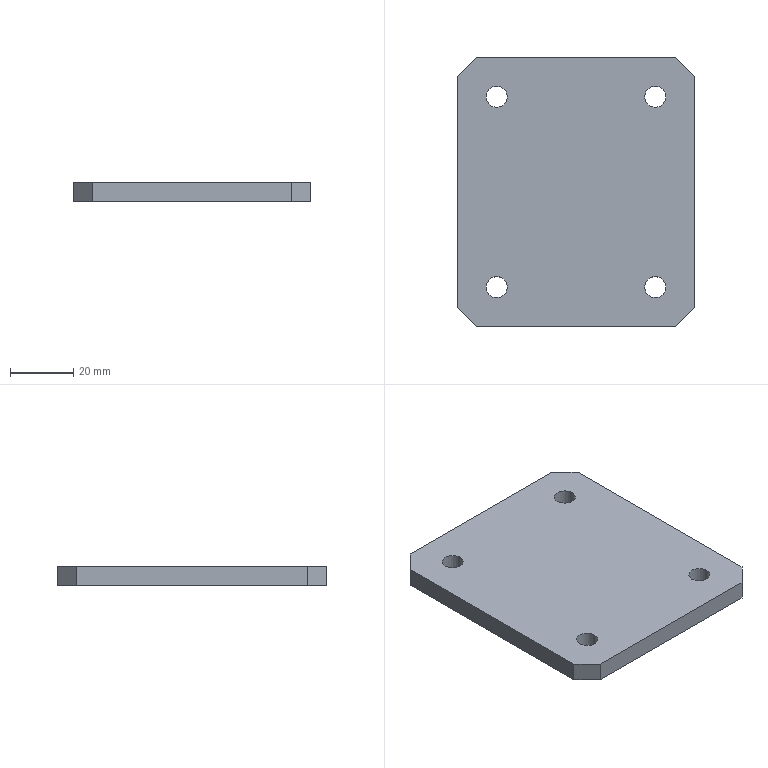Part | STEP file | linkroller | 1 solid | 14 faces | box 75 x 85 x 6 mm | volume 36985 mm3 | plane 10 | spline 4